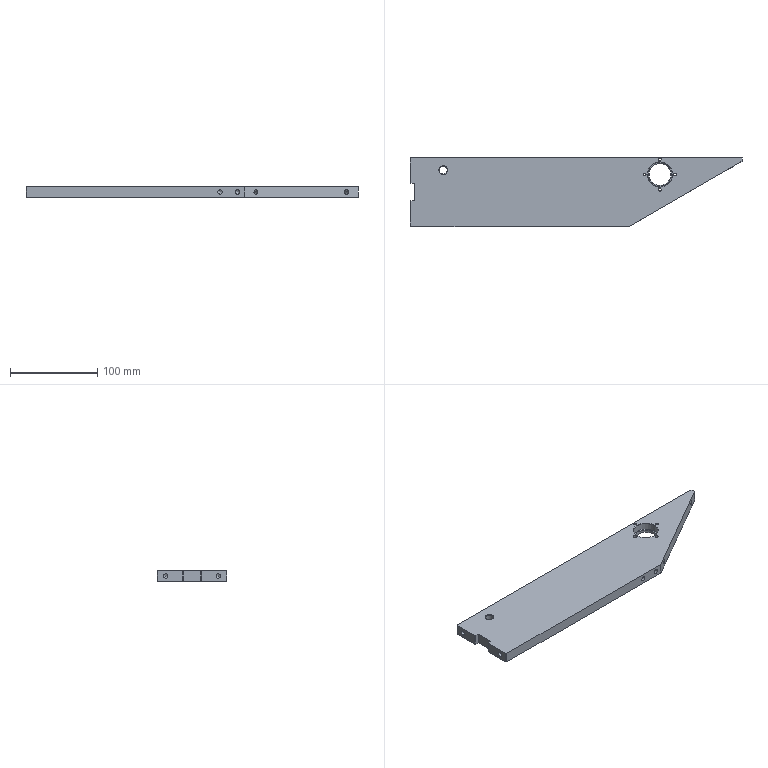CAM job | NX | 3-axis milling, drilling | part box 380 x 80 x 12 mm | stock box 384 x 80 x 12 mm
Tools:
number,name,description,diameter,corner_radius,flute_length,length,flutes
6,D8A45,Milling Tool-5 Parameters,8.0,0.0,50.0,75.0,2
12,3.3ZT,Drilling Tool,3.3,0.0,35.0,50.0,2
4,D10,Milling Tool-5 Parameters,10.0,0.0,50.0,75.0,2
22,9.0ZT,Drilling Tool,9.0,0.0,35.0,50.0,2
Operations:
program,operation,operation_type,tool,method,geometry_group,spindle_rpm,surface_speed,feed_per_tooth,feed_cut,feed_plunge,cut_length_mm,path_length_mm,cut_time_min,machine_time_min
1,DRILLING,Operation,D8A45,METHOD,A,3500.0,65.0,0.0357,250.0,0.0,28.5,447.944,0.114,0.1559
1,DRILLING_COPY,Operation,3.3ZT,METHOD,A,1500.0,15.0,0.05,150.0,0.0,69.966,283.721,0.4664,0.4878
1,DRILLING_COPY_COPY,Operation,9.0ZT,METHOD,A,1500.0,15.0,0.05,150.0,0.0,19.204,98.408,0.128,0.1359
1,ZLEVEL_PROFILE,ZLevelMilling,D10,METHOD,A,7000.0,219.0,0.2143,3000.0,1000.0,3469.994,4029.348,1.199,1.255
1,ZLEVEL_PROFILE_COPY,ZLevelMilling,D10,METHOD,A,7000.0,219.0,0.0714,1000.0,1000.0,268.221,690.987,0.2682,0.3105
1,HOLE_MILLING,CylinderMilling,D10,METHOD,A,7000.0,0.0,0.0,2000.0,100.0,839.033,915.033,0.4195,0.4271
1,HOLE_MILLING_COPY,CylinderMilling,D10,METHOD,A,7000.0,0.0,0.0893,1250.0,100.0,424.258,508.258,0.3394,0.3478
1,PLANAR_MILL,PlanarMilling,D8A45,METHOD,A,7000.0,1495.0,0.0893,1250.0,100.0,156.855,822.078,0.1255,0.192
1,PLANAR_MILL_COPY_1,PlanarMilling,D8A45,METHOD,A,7000.0,1495.0,0.0893,1250.0,100.0,263.863,634.219,0.2111,0.2481
1,刀补4,CylinderMilling,D10,METHOD,A,7000.0,0.0,0.0714,1000.0,100.0,238.315,305.815,0.2383,0.2451
NC_PROGRAM,PLANAR_MILL_COPY,PlanarMilling,D8A45,METHOD,A,7000.0,1495.0,0.0893,1250.0,100.0,0.0,0.0,0.0,0.0,missing